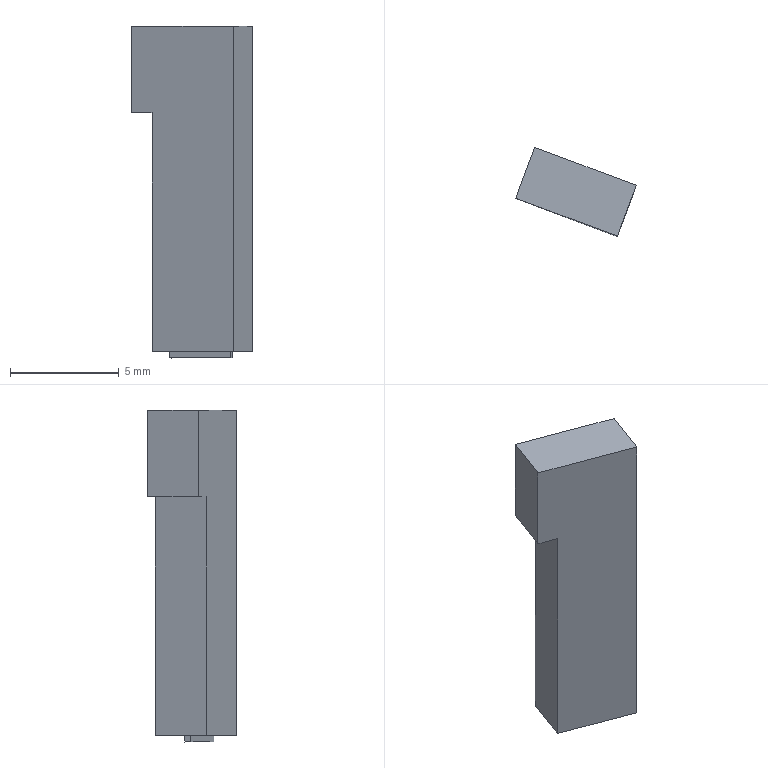Part | NX | features 13 2 | 1 solid | 18 faces | box 5.559 x 4.093 x 15.3 mm | volume 160.338 mm3 | plane 14 | spline 4